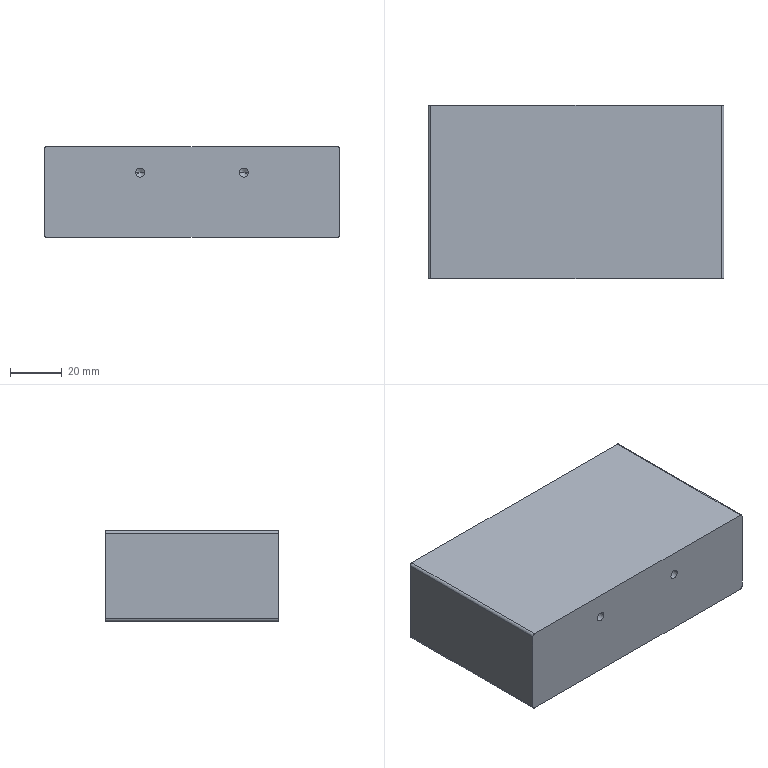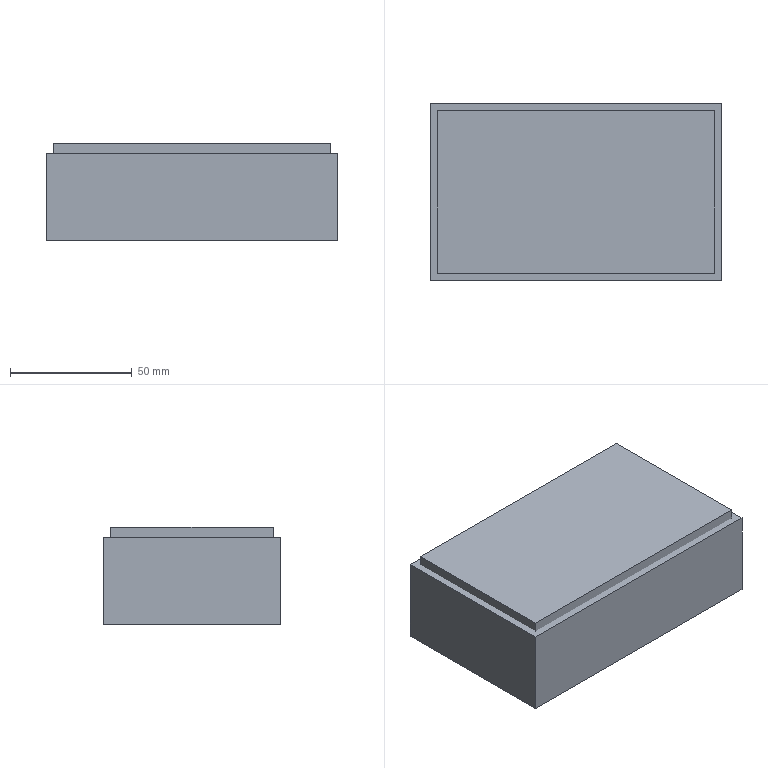CAM job | NX | 3+2 milling, drilling | part box 114 x 67 x 35 mm | stock box 120 x 73 x 40 mm
Tools:
number,name,description,diameter,corner_radius,flute_length,length,flutes
1,D63,Milling Tool-5 Parameters,63.0,0.0,50.0,75.0,2
9,D10,Milling Tool-5 Parameters,10.0,0.0,50.0,75.0,2
10,D10JING,Milling Tool-5 Parameters,10.0,0.0,50.0,75.0,2
2,D4A45,Milling Tool-5 Parameters,4.0,0.0,2.0,2.0,2
15,3.5ZT,Drilling Tool,3.5,0.0,35.0,50.0,2
Operations:
program,operation,operation_type,tool,method,geometry_group,spindle_rpm,surface_speed,feed_per_tooth,feed_cut,feed_plunge,cut_length_mm,path_length_mm,cut_time_min,machine_time_min
1,FLOOR_WALL,VolumeBased25DMillingOperation,D63,METHOD,A,6500.0,1286.0,0.0962,1250.0,100.0,608.797,662.797,0.487,0.4924
1,ZLEVEL_PROFILE,ZLevelMilling,D10,METHOD,A,9500.0,298.0,0.1579,3000.0,1000.0,13898.401,13990.401,4.665,4.674
1,ZLEVEL_PROFILE_COPY_COPY,ZLevelMilling,D10JING,METHOD,A,9500.0,119.0,0.0632,1200.0,1000.0,803.509,1025.868,0.6709,0.6932
1,ZLEVEL_PROFILE_1_COPY_1_COPY_COPY,ZLevelMilling,D4A45,METHOD,A,9500.0,179.0,0.0526,1000.0,100.0,372.683,433.683,0.3727,0.3788
2,FLOOR_WALL_COPY,VolumeBased25DMillingOperation,D63,METHOD,B,6500.0,1286.0,0.0962,1250.0,100.0,2923.985,3924.836,2.339,2.439
2,ZLEVEL_PROFILE_1_COPY_1_COPY_COPY_COPY,ZLevelMilling,D4A45,METHOD,B,9500.0,179.0,0.0526,1000.0,100.0,372.683,433.683,0.3727,0.3788
3,DRILLING_COPY,Operation,D4A45,METHOD,C,5000.0,62.0,0.025,250.0,0.0,8.0,119.112,0.032,0.0431
3,DRILLING_COPY_COPY_COPY_COPY_COPY_COPY,Operation,3.5ZT,METHOD,C,1910.0,21.0,0.0471,180.0,0.0,29.103,161.318,0.1617,0.1749
4,DRILLING_COPY_COPY,Operation,D4A45,METHOD,D,5000.0,62.0,0.025,250.0,0.0,16.0,276.3,0.064,0.09
4,DRILLING_COPY_COPY_COPY_COPY_COPY_COPY_COPY,Operation,3.5ZT,METHOD,D,1910.0,21.0,0.0471,180.0,0.0,58.206,290.797,0.3234,0.3466